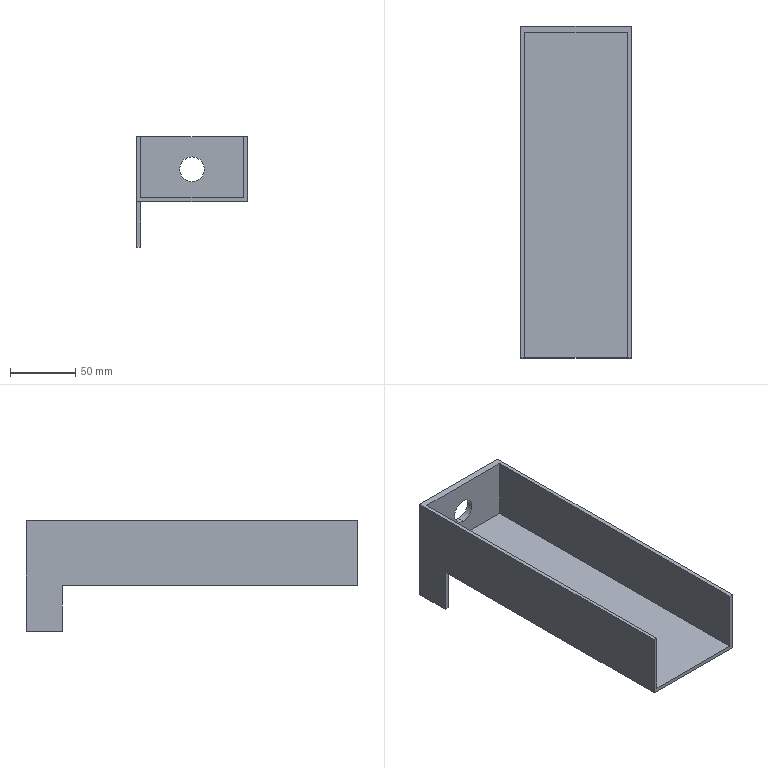Part | STEP file | Guide wheel mechanism revised.sldasm-Part-349 | 1 solid | 15 faces | box 85 x 255 x 85 mm | volume 157022 mm3 | plane 13 | cylinder 2 | commonest cylinder face diameters 19 x2
STEP:
#1=CARTESIAN_POINT('',(0.,255.,9.5));
#2=VERTEX_POINT('',#1);
#3=CARTESIAN_POINT('',(0.,255.,-9.5));
#4=VERTEX_POINT('',#3);
#5=CARTESIAN_POINT('',(0.,255.,0.));
#6=DIRECTION('',(0.,-1.,0.));
#7=DIRECTION('',(0.,0.,-1.));
#8=AXIS2_PLACEMENT_3D('',#5,#6,#7);
#9=CIRCLE('',#8,9.5);
#10=EDGE_CURVE('',#2,#4,#9,.T.);
#11=ORIENTED_EDGE('',*,*,#10,.F.);
#12=CARTESIAN_POINT('',(0.,250.,9.5));
#13=VERTEX_POINT('',#12);
#14=CARTESIAN_POINT('',(0.,255.,9.5));
#15=DIRECTION('',(0.,-1.,0.));
#16=VECTOR('',#15,1000.);
#17=LINE('',#14,#16);
#18=EDGE_CURVE('',#2,#13,#17,.T.);
#19=ORIENTED_EDGE('',*,*,#18,.T.);
#20=CARTESIAN_POINT('',(0.,250.,-9.5));
#21=VERTEX_POINT('',#20);
#22=CARTESIAN_POINT('',(0.,250.,0.));
#23=DIRECTION('',(0.,-1.,0.));
#24=DIRECTION('',(0.,0.,-1.));
#25=AXIS2_PLACEMENT_3D('',#22,#23,#24);
#26=CIRCLE('',#25,9.5);
#27=EDGE_CURVE('',#13,#21,#26,.T.);
#28=ORIENTED_EDGE('',*,*,#27,.T.);
#29=CARTESIAN_POINT('',(0.,255.,-9.5));
#30=DIRECTION('',(0.,-1.,0.));
#31=VECTOR('',#30,1000.);
#32=LINE('',#29,#31);
#33=EDGE_CURVE('',#4,#21,#32,.T.);
#34=ORIENTED_EDGE('',*,*,#33,.F.);
#35=EDGE_LOOP('',(#11,#19,#28,#34));
#36=FACE_OUTER_BOUND('',#35,.T.);
#37=CARTESIAN_POINT('',(0.,255.,0.));
#38=DIRECTION('',(0.,-1.,0.));
#39=DIRECTION('',(0.,0.,-1.));
#40=AXIS2_PLACEMENT_3D('',#37,#38,#39);
#41=CYLINDRICAL_SURFACE('',#40,9.5);
#42=ADVANCED_FACE('',(#36),#41,.F.);
#43=CARTESIAN_POINT('',(-39.5,227.,-25.));
#44=VERTEX_POINT('',#43);
#45=CARTESIAN_POINT('',(-42.5,227.,-25.));
#46=VERTEX_POINT('',#45);
#47=CARTESIAN_POINT('',(-39.5,227.,-25.));
#48=DIRECTION('',(-1.,0.,0.));
#49=VECTOR('',#48,1000.);
#50=LINE('',#47,#49);
#51=EDGE_CURVE('',#44,#46,#50,.T.);
#52=ORIENTED_EDGE('',*,*,#51,.F.);
#53=CARTESIAN_POINT('',(-39.5,255.,-25.));
#54=VERTEX_POINT('',#53);
#55=CARTESIAN_POINT('',(-39.5,255.,-25.));
#56=DIRECTION('',(0.,1.,0.));
#57=VECTOR('',#56,1000.);
#58=LINE('',#55,#57);
#59=EDGE_CURVE('',#44,#54,#58,.T.);
#60=ORIENTED_EDGE('',*,*,#59,.T.);
#61=CARTESIAN_POINT('',(42.5,255.,-25.));
#62=VERTEX_POINT('',#61);
#63=CARTESIAN_POINT('',(42.5,255.,-25.));
#64=DIRECTION('',(-1.,0.,0.));
#65=VECTOR('',#64,1000.);
#66=LINE('',#63,#65);
#67=EDGE_CURVE('',#62,#54,#66,.T.);
#68=ORIENTED_EDGE('',*,*,#67,.F.);
#69=CARTESIAN_POINT('',(42.5,0.,-25.));
#70=VERTEX_POINT('',#69);
#71=CARTESIAN_POINT('',(42.5,255.,-25.));
#72=DIRECTION('',(0.,-1.,0.));
#73=VECTOR('',#72,1000.);
#74=LINE('',#71,#73);
#75=EDGE_CURVE('',#62,#70,#74,.T.);
#76=ORIENTED_EDGE('',*,*,#75,.T.);
#77=CARTESIAN_POINT('',(-42.5,0.,-25.));
#78=VERTEX_POINT('',#77);
#79=CARTESIAN_POINT('',(42.5,0.,-25.));
#80=DIRECTION('',(-1.,0.,0.));
#81=VECTOR('',#80,1000.);
#82=LINE('',#79,#81);
#83=EDGE_CURVE('',#70,#78,#82,.T.);
#84=ORIENTED_EDGE('',*,*,#83,.T.);
#85=CARTESIAN_POINT('',(-42.5,255.,-25.));
#86=DIRECTION('',(0.,-1.,0.));
#87=VECTOR('',#86,1000.);
#88=LINE('',#85,#87);
#89=EDGE_CURVE('',#46,#78,#88,.T.);
#90=ORIENTED_EDGE('',*,*,#89,.F.);
#91=EDGE_LOOP('',(#52,#60,#68,#76,#84,#90));
#92=FACE_OUTER_BOUND('',#91,.T.);
#93=CARTESIAN_POINT('',(42.5,255.,-25.));
#94=DIRECTION('',(0.,0.,1.));
#95=DIRECTION('',(1.,0.,0.));
#96=AXIS2_PLACEMENT_3D('',#93,#94,#95);
#97=PLANE('',#96);
#98=ADVANCED_FACE('',(#92),#97,.F.);
#99=CARTESIAN_POINT('',(-42.5,0.,25.));
#100=VERTEX_POINT('',#99);
#101=CARTESIAN_POINT('',(-42.5,0.,25.));
#102=DIRECTION('',(0.,0.,1.));
#103=VECTOR('',#102,1000.);
#104=LINE('',#101,#103);
#105=EDGE_CURVE('',#78,#100,#104,.T.);
#106=ORIENTED_EDGE('',*,*,#105,.T.);
#107=CARTESIAN_POINT('',(-42.5,255.,25.));
#108=VERTEX_POINT('',#107);
#109=CARTESIAN_POINT('',(-42.5,255.,25.));
#110=DIRECTION('',(0.,-1.,0.));
#111=VECTOR('',#110,1000.);
#112=LINE('',#109,#111);
#113=EDGE_CURVE('',#108,#100,#112,.T.);
#114=ORIENTED_EDGE('',*,*,#113,.F.);
#115=CARTESIAN_POINT('',(-42.5,255.,-60.));
#116=VERTEX_POINT('',#115);
#117=CARTESIAN_POINT('',(-42.5,255.,25.));
#118=DIRECTION('',(0.,0.,1.));
#119=VECTOR('',#118,1000.);
#120=LINE('',#117,#119);
#121=EDGE_CURVE('',#116,#108,#120,.T.);
#122=ORIENTED_EDGE('',*,*,#121,.F.);
#123=CARTESIAN_POINT('',(-42.5,227.,-60.));
#124=VERTEX_POINT('',#123);
#125=CARTESIAN_POINT('',(-42.5,255.,-60.));
#126=DIRECTION('',(0.,-1.,0.));
#127=VECTOR('',#126,1000.);
#128=LINE('',#125,#127);
#129=EDGE_CURVE('',#116,#124,#128,.T.);
#130=ORIENTED_EDGE('',*,*,#129,.T.);
#131=CARTESIAN_POINT('',(-42.5,227.,-25.));
#132=DIRECTION('',(0.,0.,1.));
#133=VECTOR('',#132,1000.);
#134=LINE('',#131,#133);
#135=EDGE_CURVE('',#124,#46,#134,.T.);
#136=ORIENTED_EDGE('',*,*,#135,.T.);
#137=ORIENTED_EDGE('',*,*,#89,.T.);
#138=EDGE_LOOP('',(#106,#114,#122,#130,#136,#137));
#139=FACE_OUTER_BOUND('',#138,.T.);
#140=CARTESIAN_POINT('',(-42.5,255.,25.));
#141=DIRECTION('',(1.,0.,0.));
#142=DIRECTION('',(0.,0.,-1.));
#143=AXIS2_PLACEMENT_3D('',#140,#141,#142);
#144=PLANE('',#143);
#145=ADVANCED_FACE('',(#139),#144,.F.);
#146=CARTESIAN_POINT('',(-39.5,0.,25.));
#147=VERTEX_POINT('',#146);
#148=CARTESIAN_POINT('',(42.5,0.,25.));
#149=DIRECTION('',(1.,0.,0.));
#150=VECTOR('',#149,1000.);
#151=LINE('',#148,#150);
#152=EDGE_CURVE('',#100,#147,#151,.T.);
#153=ORIENTED_EDGE('',*,*,#152,.T.);
#154=CARTESIAN_POINT('',(-39.5,250.,25.));
#155=VERTEX_POINT('',#154);
#156=CARTESIAN_POINT('',(-39.5,250.,25.));
#157=DIRECTION('',(0.,-1.,0.));
#158=VECTOR('',#157,1000.);
#159=LINE('',#156,#158);
#160=EDGE_CURVE('',#155,#147,#159,.T.);
#161=ORIENTED_EDGE('',*,*,#160,.F.);
#162=CARTESIAN_POINT('',(39.5,250.,25.));
#163=VERTEX_POINT('',#162);
#164=CARTESIAN_POINT('',(-39.5,250.,25.));
#165=DIRECTION('',(-1.,0.,0.));
#166=VECTOR('',#165,1000.);
#167=LINE('',#164,#166);
#168=EDGE_CURVE('',#163,#155,#167,.T.);
#169=ORIENTED_EDGE('',*,*,#168,.F.);
#170=CARTESIAN_POINT('',(39.5,0.,25.));
#171=VERTEX_POINT('',#170);
#172=CARTESIAN_POINT('',(39.5,250.,25.));
#173=DIRECTION('',(0.,-1.,0.));
#174=VECTOR('',#173,1000.);
#175=LINE('',#172,#174);
#176=EDGE_CURVE('',#163,#171,#175,.T.);
#177=ORIENTED_EDGE('',*,*,#176,.T.);
#178=CARTESIAN_POINT('',(42.5,0.,25.));
#179=VERTEX_POINT('',#178);
#180=CARTESIAN_POINT('',(42.5,0.,25.));
#181=DIRECTION('',(1.,0.,0.));
#182=VECTOR('',#181,1000.);
#183=LINE('',#180,#182);
#184=EDGE_CURVE('',#171,#179,#183,.T.);
#185=ORIENTED_EDGE('',*,*,#184,.T.);
#186=CARTESIAN_POINT('',(42.5,255.,25.));
#187=VERTEX_POINT('',#186);
#188=CARTESIAN_POINT('',(42.5,255.,25.));
#189=DIRECTION('',(0.,-1.,0.));
#190=VECTOR('',#189,1000.);
#191=LINE('',#188,#190);
#192=EDGE_CURVE('',#187,#179,#191,.T.);
#193=ORIENTED_EDGE('',*,*,#192,.F.);
#194=CARTESIAN_POINT('',(42.5,255.,25.));
#195=DIRECTION('',(1.,0.,0.));
#196=VECTOR('',#195,1000.);
#197=LINE('',#194,#196);
#198=EDGE_CURVE('',#108,#187,#197,.T.);
#199=ORIENTED_EDGE('',*,*,#198,.F.);
#200=ORIENTED_EDGE('',*,*,#113,.T.);
#201=EDGE_LOOP('',(#153,#161,#169,#177,#185,#193,#199,#200));
#202=FACE_OUTER_BOUND('',#201,.T.);
#203=CARTESIAN_POINT('',(42.5,255.,25.));
#204=DIRECTION('',(0.,0.,-1.));
#205=DIRECTION('',(-1.,0.,0.));
#206=AXIS2_PLACEMENT_3D('',#203,#204,#205);
#207=PLANE('',#206);
#208=ADVANCED_FACE('',(#202),#207,.F.);
#209=CARTESIAN_POINT('',(42.5,0.,25.));
#210=DIRECTION('',(0.,0.,-1.));
#211=VECTOR('',#210,1000.);
#212=LINE('',#209,#211);
#213=EDGE_CURVE('',#179,#70,#212,.T.);
#214=ORIENTED_EDGE('',*,*,#213,.T.);
#215=ORIENTED_EDGE('',*,*,#75,.F.);
#216=CARTESIAN_POINT('',(42.5,255.,25.));
#217=DIRECTION('',(0.,0.,-1.));
#218=VECTOR('',#217,1000.);
#219=LINE('',#216,#218);
#220=EDGE_CURVE('',#187,#62,#219,.T.);
#221=ORIENTED_EDGE('',*,*,#220,.F.);
#222=ORIENTED_EDGE('',*,*,#192,.T.);
#223=EDGE_LOOP('',(#214,#215,#221,#222));
#224=FACE_OUTER_BOUND('',#223,.T.);
#225=CARTESIAN_POINT('',(42.5,255.,25.));
#226=DIRECTION('',(-1.,0.,0.));
#227=DIRECTION('',(0.,0.,1.));
#228=AXIS2_PLACEMENT_3D('',#225,#226,#227);
#229=PLANE('',#228);
#230=ADVANCED_FACE('',(#224),#229,.F.);
#231=CARTESIAN_POINT('',(0.,255.,0.));
#232=DIRECTION('',(0.,-1.,0.));
#233=DIRECTION('',(0.,0.,-1.));
#234=AXIS2_PLACEMENT_3D('',#231,#232,#233);
#235=CIRCLE('',#234,9.5);
#236=EDGE_CURVE('',#4,#2,#235,.T.);
#237=ORIENTED_EDGE('',*,*,#236,.T.);
#238=ORIENTED_EDGE('',*,*,#10,.T.);
#239=EDGE_LOOP('',(#237,#238));
#240=FACE_BOUND('',#239,.T.);
#241=ORIENTED_EDGE('',*,*,#121,.T.);
#242=ORIENTED_EDGE('',*,*,#198,.T.);
#243=ORIENTED_EDGE('',*,*,#220,.T.);
#244=ORIENTED_EDGE('',*,*,#67,.T.);
#245=CARTESIAN_POINT('',(-39.5,255.,-60.));
#246=VERTEX_POINT('',#245);
#247=CARTESIAN_POINT('',(-39.5,255.,-25.));
#248=DIRECTION('',(0.,0.,-1.));
#249=VECTOR('',#248,1000.);
#250=LINE('',#247,#249);
#251=EDGE_CURVE('',#54,#246,#250,.T.);
#252=ORIENTED_EDGE('',*,*,#251,.T.);
#253=CARTESIAN_POINT('',(-39.5,255.,-60.));
#254=DIRECTION('',(-1.,0.,0.));
#255=VECTOR('',#254,1000.);
#256=LINE('',#253,#255);
#257=EDGE_CURVE('',#246,#116,#256,.T.);
#258=ORIENTED_EDGE('',*,*,#257,.T.);
#259=EDGE_LOOP('',(#241,#242,#243,#244,#252,#258));
#260=FACE_OUTER_BOUND('',#259,.T.);
#261=CARTESIAN_POINT('',(0.,255.,0.));
#262=DIRECTION('',(0.,1.,0.));
#263=DIRECTION('',(0.,0.,1.));
#264=AXIS2_PLACEMENT_3D('',#261,#262,#263);
#265=PLANE('',#264);
#266=ADVANCED_FACE('',(#240,#260),#265,.T.);
#267=CARTESIAN_POINT('',(-39.5,0.,-22.));
#268=VERTEX_POINT('',#267);
#269=CARTESIAN_POINT('',(39.5,0.,-22.));
#270=VERTEX_POINT('',#269);
#271=CARTESIAN_POINT('',(-39.5,0.,-22.));
#272=DIRECTION('',(1.,0.,0.));
#273=VECTOR('',#272,1000.);
#274=LINE('',#271,#273);
#275=EDGE_CURVE('',#268,#270,#274,.T.);
#276=ORIENTED_EDGE('',*,*,#275,.F.);
#277=CARTESIAN_POINT('',(-39.5,0.,25.));
#278=DIRECTION('',(0.,0.,-1.));
#279=VECTOR('',#278,1000.);
#280=LINE('',#277,#279);
#281=EDGE_CURVE('',#147,#268,#280,.T.);
#282=ORIENTED_EDGE('',*,*,#281,.F.);
#283=ORIENTED_EDGE('',*,*,#152,.F.);
#284=ORIENTED_EDGE('',*,*,#105,.F.);
#285=ORIENTED_EDGE('',*,*,#83,.F.);
#286=ORIENTED_EDGE('',*,*,#213,.F.);
#287=ORIENTED_EDGE('',*,*,#184,.F.);
#288=CARTESIAN_POINT('',(39.5,0.,25.));
#289=DIRECTION('',(0.,0.,1.));
#290=VECTOR('',#289,1000.);
#291=LINE('',#288,#290);
#292=EDGE_CURVE('',#270,#171,#291,.T.);
#293=ORIENTED_EDGE('',*,*,#292,.F.);
#294=EDGE_LOOP('',(#276,#282,#283,#284,#285,#286,#287,#293));
#295=FACE_OUTER_BOUND('',#294,.T.);
#296=CARTESIAN_POINT('',(0.,0.,0.));
#297=DIRECTION('',(0.,1.,0.));
#298=DIRECTION('',(0.,0.,1.));
#299=AXIS2_PLACEMENT_3D('',#296,#297,#298);
#300=PLANE('',#299);
#301=ADVANCED_FACE('',(#295),#300,.F.);
#302=ORIENTED_EDGE('',*,*,#281,.T.);
#303=CARTESIAN_POINT('',(-39.5,250.,-22.));
#304=VERTEX_POINT('',#303);
#305=CARTESIAN_POINT('',(-39.5,250.,-22.));
#306=DIRECTION('',(0.,-1.,0.));
#307=VECTOR('',#306,1000.);
#308=LINE('',#305,#307);
#309=EDGE_CURVE('',#304,#268,#308,.T.);
#310=ORIENTED_EDGE('',*,*,#309,.F.);
#311=CARTESIAN_POINT('',(-39.5,250.,25.));
#312=DIRECTION('',(0.,0.,-1.));
#313=VECTOR('',#312,1000.);
#314=LINE('',#311,#313);
#315=EDGE_CURVE('',#155,#304,#314,.T.);
#316=ORIENTED_EDGE('',*,*,#315,.F.);
#317=ORIENTED_EDGE('',*,*,#160,.T.);
#318=EDGE_LOOP('',(#302,#310,#316,#317));
#319=FACE_OUTER_BOUND('',#318,.T.);
#320=CARTESIAN_POINT('',(-39.5,250.,25.));
#321=DIRECTION('',(-1.,0.,0.));
#322=DIRECTION('',(0.,0.,1.));
#323=AXIS2_PLACEMENT_3D('',#320,#321,#322);
#324=PLANE('',#323);
#325=ADVANCED_FACE('',(#319),#324,.F.);
#326=ORIENTED_EDGE('',*,*,#292,.T.);
#327=ORIENTED_EDGE('',*,*,#176,.F.);
#328=CARTESIAN_POINT('',(39.5,250.,-22.));
#329=VERTEX_POINT('',#328);
#330=CARTESIAN_POINT('',(39.5,250.,25.));
#331=DIRECTION('',(0.,0.,1.));
#332=VECTOR('',#331,1000.);
#333=LINE('',#330,#332);
#334=EDGE_CURVE('',#329,#163,#333,.T.);
#335=ORIENTED_EDGE('',*,*,#334,.F.);
#336=CARTESIAN_POINT('',(39.5,250.,-22.));
#337=DIRECTION('',(0.,-1.,0.));
#338=VECTOR('',#337,1000.);
#339=LINE('',#336,#338);
#340=EDGE_CURVE('',#329,#270,#339,.T.);
#341=ORIENTED_EDGE('',*,*,#340,.T.);
#342=EDGE_LOOP('',(#326,#327,#335,#341));
#343=FACE_OUTER_BOUND('',#342,.T.);
#344=CARTESIAN_POINT('',(39.5,250.,25.));
#345=DIRECTION('',(1.,0.,0.));
#346=DIRECTION('',(0.,0.,-1.));
#347=AXIS2_PLACEMENT_3D('',#344,#345,#346);
#348=PLANE('',#347);
#349=ADVANCED_FACE('',(#343),#348,.F.);
#350=ORIENTED_EDGE('',*,*,#275,.T.);
#351=ORIENTED_EDGE('',*,*,#340,.F.);
#352=CARTESIAN_POINT('',(-39.5,250.,-22.));
#353=DIRECTION('',(1.,0.,0.));
#354=VECTOR('',#353,1000.);
#355=LINE('',#352,#354);
#356=EDGE_CURVE('',#304,#329,#355,.T.);
#357=ORIENTED_EDGE('',*,*,#356,.F.);
#358=ORIENTED_EDGE('',*,*,#309,.T.);
#359=EDGE_LOOP('',(#350,#351,#357,#358));
#360=FACE_OUTER_BOUND('',#359,.T.);
#361=CARTESIAN_POINT('',(-39.5,250.,-22.));
#362=DIRECTION('',(0.,0.,-1.));
#363=DIRECTION('',(-1.,0.,0.));
#364=AXIS2_PLACEMENT_3D('',#361,#362,#363);
#365=PLANE('',#364);
#366=ADVANCED_FACE('',(#360),#365,.F.);
#367=CARTESIAN_POINT('',(0.,250.,0.));
#368=DIRECTION('',(0.,-1.,0.));
#369=DIRECTION('',(0.,0.,-1.));
#370=AXIS2_PLACEMENT_3D('',#367,#368,#369);
#371=CIRCLE('',#370,9.5);
#372=EDGE_CURVE('',#21,#13,#371,.T.);
#373=ORIENTED_EDGE('',*,*,#372,.F.);
#374=ORIENTED_EDGE('',*,*,#27,.F.);
#375=EDGE_LOOP('',(#373,#374));
#376=FACE_BOUND('',#375,.T.);
#377=ORIENTED_EDGE('',*,*,#315,.T.);
#378=ORIENTED_EDGE('',*,*,#356,.T.);
#379=ORIENTED_EDGE('',*,*,#334,.T.);
#380=ORIENTED_EDGE('',*,*,#168,.T.);
#381=EDGE_LOOP('',(#377,#378,#379,#380));
#382=FACE_OUTER_BOUND('',#381,.T.);
#383=CARTESIAN_POINT('',(0.,250.,0.));
#384=DIRECTION('',(0.,-1.,0.));
#385=DIRECTION('',(0.,0.,-1.));
#386=AXIS2_PLACEMENT_3D('',#383,#384,#385);
#387=PLANE('',#386);
#388=ADVANCED_FACE('',(#376,#382),#387,.T.);
#389=ORIENTED_EDGE('',*,*,#18,.F.);
#390=ORIENTED_EDGE('',*,*,#236,.F.);
#391=ORIENTED_EDGE('',*,*,#33,.T.);
#392=ORIENTED_EDGE('',*,*,#372,.T.);
#393=EDGE_LOOP('',(#389,#390,#391,#392));
#394=FACE_OUTER_BOUND('',#393,.T.);
#395=CARTESIAN_POINT('',(0.,255.,0.));
#396=DIRECTION('',(0.,-1.,0.));
#397=DIRECTION('',(0.,0.,-1.));
#398=AXIS2_PLACEMENT_3D('',#395,#396,#397);
#399=CYLINDRICAL_SURFACE('',#398,9.5);
#400=ADVANCED_FACE('',(#394),#399,.F.);
#401=ORIENTED_EDGE('',*,*,#135,.F.);
#402=CARTESIAN_POINT('',(-39.5,227.,-60.));
#403=VERTEX_POINT('',#402);
#404=CARTESIAN_POINT('',(-39.5,227.,-60.));
#405=DIRECTION('',(-1.,0.,0.));
#406=VECTOR('',#405,1000.);
#407=LINE('',#404,#406);
#408=EDGE_CURVE('',#403,#124,#407,.T.);
#409=ORIENTED_EDGE('',*,*,#408,.F.);
#410=CARTESIAN_POINT('',(-39.5,227.,-25.));
#411=DIRECTION('',(0.,0.,1.));
#412=VECTOR('',#411,1000.);
#413=LINE('',#410,#412);
#414=EDGE_CURVE('',#403,#44,#413,.T.);
#415=ORIENTED_EDGE('',*,*,#414,.T.);
#416=ORIENTED_EDGE('',*,*,#51,.T.);
#417=EDGE_LOOP('',(#401,#409,#415,#416));
#418=FACE_OUTER_BOUND('',#417,.T.);
#419=CARTESIAN_POINT('',(-39.5,227.,-25.));
#420=DIRECTION('',(0.,-1.,0.));
#421=DIRECTION('',(0.,0.,-1.));
#422=AXIS2_PLACEMENT_3D('',#419,#420,#421);
#423=PLANE('',#422);
#424=ADVANCED_FACE('',(#418),#423,.T.);
#425=ORIENTED_EDGE('',*,*,#129,.F.);
#426=ORIENTED_EDGE('',*,*,#257,.F.);
#427=CARTESIAN_POINT('',(-39.5,255.,-60.));
#428=DIRECTION('',(0.,-1.,0.));
#429=VECTOR('',#428,1000.);
#430=LINE('',#427,#429);
#431=EDGE_CURVE('',#246,#403,#430,.T.);
#432=ORIENTED_EDGE('',*,*,#431,.T.);
#433=ORIENTED_EDGE('',*,*,#408,.T.);
#434=EDGE_LOOP('',(#425,#426,#432,#433));
#435=FACE_OUTER_BOUND('',#434,.T.);
#436=CARTESIAN_POINT('',(-39.5,255.,-60.));
#437=DIRECTION('',(0.,0.,-1.));
#438=DIRECTION('',(-1.,0.,0.));
#439=AXIS2_PLACEMENT_3D('',#436,#437,#438);
#440=PLANE('',#439);
#441=ADVANCED_FACE('',(#435),#440,.T.);
#442=ORIENTED_EDGE('',*,*,#59,.F.);
#443=ORIENTED_EDGE('',*,*,#414,.F.);
#444=ORIENTED_EDGE('',*,*,#431,.F.);
#445=ORIENTED_EDGE('',*,*,#251,.F.);
#446=EDGE_LOOP('',(#442,#443,#444,#445));
#447=FACE_OUTER_BOUND('',#446,.T.);
#448=CARTESIAN_POINT('',(-39.5,0.,0.));
#449=DIRECTION('',(1.,0.,0.));
#450=DIRECTION('',(0.,0.,-1.));
#451=AXIS2_PLACEMENT_3D('',#448,#449,#450);
#452=PLANE('',#451);
#453=ADVANCED_FACE('',(#447),#452,.T.);
#454=CLOSED_SHELL('',(#42,#98,#145,#208,#230,#266,#301,#325,#349,#366,#388,#400,#424,#441,#453));
#455=MANIFOLD_SOLID_BREP('',#454);
#456=CARTESIAN_POINT('',(0.,0.,0.));
#457=DIRECTION('',(0.,0.,1.));
#458=DIRECTION('',(1.,0.,0.));
#459=AXIS2_PLACEMENT_3D('',#456,#457,#458);
#460=(LENGTH_UNIT()NAMED_UNIT(*)SI_UNIT(.MILLI.,.METRE.));
#461=UNCERTAINTY_MEASURE_WITH_UNIT(LENGTH_MEASURE(0.00001),#460,'','');
#462=(NAMED_UNIT(*)PLANE_ANGLE_UNIT()SI_UNIT($,.RADIAN.));
#463=(NAMED_UNIT(*)SI_UNIT($,.STERADIAN.)SOLID_ANGLE_UNIT());
#464=(GEOMETRIC_REPRESENTATION_CONTEXT(3)GLOBAL_UNCERTAINTY_ASSIGNED_CONTEXT((#461))GLOBAL_UNIT_ASSIGNED_CONTEXT((#460,#462,#463))REPRESENTATION_CONTEXT('',''));
#465=ADVANCED_BREP_SHAPE_REPRESENTATION('',(#455,#459),#464);